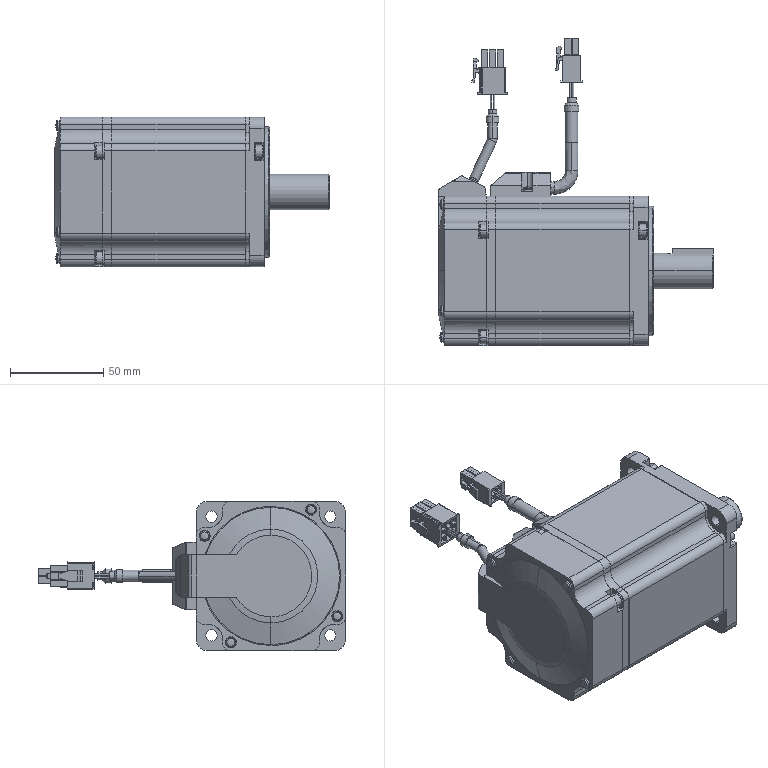Part | SolidWorks | features BaseBody 7 | 7 solids | 992 faces | box 147.2 x 164.554 x 80 mm | volume 672337 mm3 | plane 585 | cylinder 305 | cone 64 | spline 34 | torus 4 | commonest cylinder face diameters 8 x48 1 x35 2.6 x26 6 x20 7.84 x20 7 x18